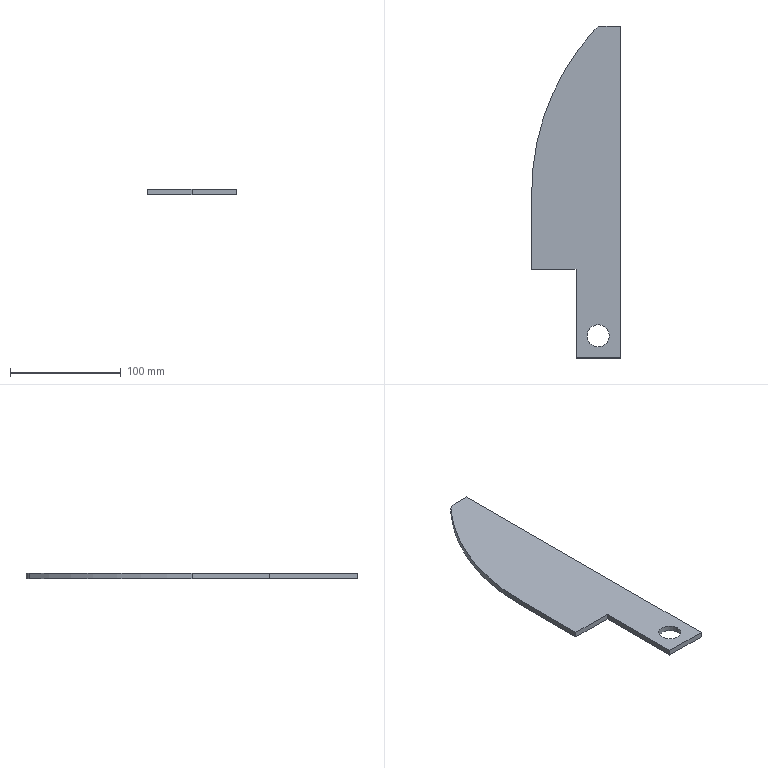Part | STEP file | qianjiaozheban | 1 solid | 11 faces | box 80 x 300 x 5 mm | volume 88356 mm3 | plane 8 | cylinder 3 | commonest cylinder face diameters 20 x2 435 x1
STEP:
#1=CARTESIAN_POINT('',(0.,0.,0.));
#2=DIRECTION('',(0.,0.,1.));
#3=DIRECTION('',(1.,0.,0.));
#4=AXIS2_PLACEMENT_3D('',#1,#2,#3);
#5=CARTESIAN_POINT('',(0.,80.,-2.5));
#6=VERTEX_POINT('',#5);
#7=CARTESIAN_POINT('',(0.,0.,-2.5));
#8=VERTEX_POINT('',#7);
#9=CARTESIAN_POINT('',(0.,0.,-2.5));
#10=DIRECTION('',(0.,-1.,0.));
#11=VECTOR('',#10,1.);
#12=LINE('',#9,#11);
#13=CARTESIAN_POINT('',(0.,0.,2.5));
#14=DIRECTION('',(1.,0.,0.));
#15=DIRECTION('',(0.,0.,-1.));
#16=AXIS2_PLACEMENT_3D('',#13,#14,#15);
#17=PLANE('',#16);
#18=CARTESIAN_POINT('',(5.,0.));
#19=DIRECTION('',(0.,-1.));
#20=VECTOR('',#19,1.);
#21=LINE('',#18,#20);
#22=(GEOMETRIC_REPRESENTATION_CONTEXT(2)PARAMETRIC_REPRESENTATION_CONTEXT()REPRESENTATION_CONTEXT('',''));
#23=DEFINITIONAL_REPRESENTATION('',(#21),#22);
#24=PCURVE('',#17,#23);
#25=CARTESIAN_POINT('',(177.5,150.,-2.5));
#26=DIRECTION('',(0.,0.,-1.));
#27=DIRECTION('',(-1.,0.,0.));
#28=AXIS2_PLACEMENT_3D('',#25,#26,#27);
#29=PLANE('',#28);
#30=CARTESIAN_POINT('',(177.5,-150.));
#31=DIRECTION('',(0.,-1.));
#32=VECTOR('',#31,1.);
#33=LINE('',#30,#32);
#34=(GEOMETRIC_REPRESENTATION_CONTEXT(2)PARAMETRIC_REPRESENTATION_CONTEXT()REPRESENTATION_CONTEXT('',''));
#35=DEFINITIONAL_REPRESENTATION('',(#33),#34);
#36=PCURVE('',#29,#35);
#37=SURFACE_CURVE('',#12,(#24,#36),.PCURVE_S1.);
#38=EDGE_CURVE('',#6,#8,#37,.T.);
#39=ORIENTED_EDGE('',*,*,#38,.T.);
#40=CARTESIAN_POINT('',(0.,0.,2.5));
#41=VERTEX_POINT('',#40);
#42=CARTESIAN_POINT('',(0.,0.,2.5));
#43=DIRECTION('',(0.,0.,-1.));
#44=VECTOR('',#43,1.);
#45=LINE('',#42,#44);
#46=CARTESIAN_POINT('',(0.,0.));
#47=DIRECTION('',(1.,0.));
#48=VECTOR('',#47,1.);
#49=LINE('',#46,#48);
#50=(GEOMETRIC_REPRESENTATION_CONTEXT(2)PARAMETRIC_REPRESENTATION_CONTEXT()REPRESENTATION_CONTEXT('',''));
#51=DEFINITIONAL_REPRESENTATION('',(#49),#50);
#52=PCURVE('',#17,#51);
#53=CARTESIAN_POINT('',(0.,0.,2.5));
#54=DIRECTION('',(0.,1.,0.));
#55=DIRECTION('',(0.,0.,1.));
#56=AXIS2_PLACEMENT_3D('',#53,#54,#55);
#57=PLANE('',#56);
#58=CARTESIAN_POINT('',(0.,0.));
#59=DIRECTION('',(-1.,0.));
#60=VECTOR('',#59,1.);
#61=LINE('',#58,#60);
#62=(GEOMETRIC_REPRESENTATION_CONTEXT(2)PARAMETRIC_REPRESENTATION_CONTEXT()REPRESENTATION_CONTEXT('',''));
#63=DEFINITIONAL_REPRESENTATION('',(#61),#62);
#64=PCURVE('',#57,#63);
#65=SURFACE_CURVE('',#45,(#52,#64),.PCURVE_S1.);
#66=EDGE_CURVE('',#41,#8,#65,.T.);
#67=ORIENTED_EDGE('',*,*,#66,.F.);
#68=CARTESIAN_POINT('',(0.,80.,2.5));
#69=VERTEX_POINT('',#68);
#70=CARTESIAN_POINT('',(0.,0.,2.5));
#71=DIRECTION('',(0.,-1.,0.));
#72=VECTOR('',#71,1.);
#73=LINE('',#70,#72);
#74=CARTESIAN_POINT('',(0.,0.));
#75=DIRECTION('',(0.,-1.));
#76=VECTOR('',#75,1.);
#77=LINE('',#74,#76);
#78=(GEOMETRIC_REPRESENTATION_CONTEXT(2)PARAMETRIC_REPRESENTATION_CONTEXT()REPRESENTATION_CONTEXT('',''));
#79=DEFINITIONAL_REPRESENTATION('',(#77),#78);
#80=PCURVE('',#17,#79);
#81=CARTESIAN_POINT('',(177.5,150.,2.5));
#82=DIRECTION('',(0.,0.,-1.));
#83=DIRECTION('',(-1.,0.,0.));
#84=AXIS2_PLACEMENT_3D('',#81,#82,#83);
#85=PLANE('',#84);
#86=CARTESIAN_POINT('',(177.5,-150.));
#87=DIRECTION('',(0.,-1.));
#88=VECTOR('',#87,1.);
#89=LINE('',#86,#88);
#90=(GEOMETRIC_REPRESENTATION_CONTEXT(2)PARAMETRIC_REPRESENTATION_CONTEXT()REPRESENTATION_CONTEXT('',''));
#91=DEFINITIONAL_REPRESENTATION('',(#89),#90);
#92=PCURVE('',#85,#91);
#93=SURFACE_CURVE('',#73,(#80,#92),.PCURVE_S1.);
#94=EDGE_CURVE('',#69,#41,#93,.T.);
#95=ORIENTED_EDGE('',*,*,#94,.F.);
#96=CARTESIAN_POINT('',(0.,80.,2.5));
#97=DIRECTION('',(0.,0.,-1.));
#98=VECTOR('',#97,1.);
#99=LINE('',#96,#98);
#100=CARTESIAN_POINT('',(0.,80.));
#101=DIRECTION('',(1.,0.));
#102=VECTOR('',#101,1.);
#103=LINE('',#100,#102);
#104=(GEOMETRIC_REPRESENTATION_CONTEXT(2)PARAMETRIC_REPRESENTATION_CONTEXT()REPRESENTATION_CONTEXT('',''));
#105=DEFINITIONAL_REPRESENTATION('',(#103),#104);
#106=PCURVE('',#17,#105);
#107=CARTESIAN_POINT('',(0.,80.,2.5));
#108=DIRECTION('',(0.,1.,0.));
#109=DIRECTION('',(0.,0.,1.));
#110=AXIS2_PLACEMENT_3D('',#107,#108,#109);
#111=PLANE('',#110);
#112=CARTESIAN_POINT('',(0.,0.));
#113=DIRECTION('',(-1.,0.));
#114=VECTOR('',#113,1.);
#115=LINE('',#112,#114);
#116=(GEOMETRIC_REPRESENTATION_CONTEXT(2)PARAMETRIC_REPRESENTATION_CONTEXT()REPRESENTATION_CONTEXT('',''));
#117=DEFINITIONAL_REPRESENTATION('',(#115),#116);
#118=PCURVE('',#111,#117);
#119=SURFACE_CURVE('',#99,(#106,#118),.PCURVE_S1.);
#120=EDGE_CURVE('',#69,#6,#119,.T.);
#121=ORIENTED_EDGE('',*,*,#120,.T.);
#122=EDGE_LOOP('',(#39,#67,#95,#121));
#123=FACE_BOUND('',#122,.T.);
#124=ADVANCED_FACE('',(#123),#17,.F.);
#125=CARTESIAN_POINT('',(40.,0.,-2.5));
#126=VERTEX_POINT('',#125);
#127=CARTESIAN_POINT('',(0.,0.,-2.5));
#128=DIRECTION('',(1.,0.,0.));
#129=VECTOR('',#128,1.);
#130=LINE('',#127,#129);
#131=CARTESIAN_POINT('',(-5.,0.));
#132=DIRECTION('',(0.,1.));
#133=VECTOR('',#132,1.);
#134=LINE('',#131,#133);
#135=(GEOMETRIC_REPRESENTATION_CONTEXT(2)PARAMETRIC_REPRESENTATION_CONTEXT()REPRESENTATION_CONTEXT('',''));
#136=DEFINITIONAL_REPRESENTATION('',(#134),#135);
#137=PCURVE('',#57,#136);
#138=CARTESIAN_POINT('',(177.5,-150.));
#139=DIRECTION('',(-1.,0.));
#140=VECTOR('',#139,1.);
#141=LINE('',#138,#140);
#142=(GEOMETRIC_REPRESENTATION_CONTEXT(2)PARAMETRIC_REPRESENTATION_CONTEXT()REPRESENTATION_CONTEXT('',''));
#143=DEFINITIONAL_REPRESENTATION('',(#141),#142);
#144=PCURVE('',#29,#143);
#145=SURFACE_CURVE('',#130,(#137,#144),.PCURVE_S1.);
#146=EDGE_CURVE('',#8,#126,#145,.T.);
#147=ORIENTED_EDGE('',*,*,#146,.T.);
#148=CARTESIAN_POINT('',(40.,0.,2.5));
#149=VERTEX_POINT('',#148);
#150=CARTESIAN_POINT('',(40.,0.,2.5));
#151=DIRECTION('',(0.,0.,-1.));
#152=VECTOR('',#151,1.);
#153=LINE('',#150,#152);
#154=CARTESIAN_POINT('',(0.,40.));
#155=DIRECTION('',(-1.,0.));
#156=VECTOR('',#155,1.);
#157=LINE('',#154,#156);
#158=(GEOMETRIC_REPRESENTATION_CONTEXT(2)PARAMETRIC_REPRESENTATION_CONTEXT()REPRESENTATION_CONTEXT('',''));
#159=DEFINITIONAL_REPRESENTATION('',(#157),#158);
#160=PCURVE('',#57,#159);
#161=CARTESIAN_POINT('',(40.,0.,2.5));
#162=DIRECTION('',(-1.,0.,0.));
#163=DIRECTION('',(0.,0.,1.));
#164=AXIS2_PLACEMENT_3D('',#161,#162,#163);
#165=PLANE('',#164);
#166=CARTESIAN_POINT('',(0.,0.));
#167=DIRECTION('',(-1.,0.));
#168=VECTOR('',#167,1.);
#169=LINE('',#166,#168);
#170=(GEOMETRIC_REPRESENTATION_CONTEXT(2)PARAMETRIC_REPRESENTATION_CONTEXT()REPRESENTATION_CONTEXT('',''));
#171=DEFINITIONAL_REPRESENTATION('',(#169),#170);
#172=PCURVE('',#165,#171);
#173=SURFACE_CURVE('',#153,(#160,#172),.PCURVE_S1.);
#174=EDGE_CURVE('',#149,#126,#173,.T.);
#175=ORIENTED_EDGE('',*,*,#174,.F.);
#176=CARTESIAN_POINT('',(0.,0.,2.5));
#177=DIRECTION('',(1.,0.,0.));
#178=VECTOR('',#177,1.);
#179=LINE('',#176,#178);
#180=CARTESIAN_POINT('',(0.,0.));
#181=DIRECTION('',(0.,1.));
#182=VECTOR('',#181,1.);
#183=LINE('',#180,#182);
#184=(GEOMETRIC_REPRESENTATION_CONTEXT(2)PARAMETRIC_REPRESENTATION_CONTEXT()REPRESENTATION_CONTEXT('',''));
#185=DEFINITIONAL_REPRESENTATION('',(#183),#184);
#186=PCURVE('',#57,#185);
#187=CARTESIAN_POINT('',(177.5,-150.));
#188=DIRECTION('',(-1.,0.));
#189=VECTOR('',#188,1.);
#190=LINE('',#187,#189);
#191=(GEOMETRIC_REPRESENTATION_CONTEXT(2)PARAMETRIC_REPRESENTATION_CONTEXT()REPRESENTATION_CONTEXT('',''));
#192=DEFINITIONAL_REPRESENTATION('',(#190),#191);
#193=PCURVE('',#85,#192);
#194=SURFACE_CURVE('',#179,(#186,#193),.PCURVE_S1.);
#195=EDGE_CURVE('',#41,#149,#194,.T.);
#196=ORIENTED_EDGE('',*,*,#195,.F.);
#197=ORIENTED_EDGE('',*,*,#66,.T.);
#198=EDGE_LOOP('',(#147,#175,#196,#197));
#199=FACE_BOUND('',#198,.T.);
#200=ADVANCED_FACE('',(#199),#57,.F.);
#201=CARTESIAN_POINT('',(40.,300.,-2.5));
#202=VERTEX_POINT('',#201);
#203=CARTESIAN_POINT('',(40.,0.,-2.5));
#204=DIRECTION('',(0.,1.,0.));
#205=VECTOR('',#204,1.);
#206=LINE('',#203,#205);
#207=CARTESIAN_POINT('',(-5.,0.));
#208=DIRECTION('',(0.,1.));
#209=VECTOR('',#208,1.);
#210=LINE('',#207,#209);
#211=(GEOMETRIC_REPRESENTATION_CONTEXT(2)PARAMETRIC_REPRESENTATION_CONTEXT()REPRESENTATION_CONTEXT('',''));
#212=DEFINITIONAL_REPRESENTATION('',(#210),#211);
#213=PCURVE('',#165,#212);
#214=CARTESIAN_POINT('',(137.5,-150.));
#215=DIRECTION('',(0.,1.));
#216=VECTOR('',#215,1.);
#217=LINE('',#214,#216);
#218=(GEOMETRIC_REPRESENTATION_CONTEXT(2)PARAMETRIC_REPRESENTATION_CONTEXT()REPRESENTATION_CONTEXT('',''));
#219=DEFINITIONAL_REPRESENTATION('',(#217),#218);
#220=PCURVE('',#29,#219);
#221=SURFACE_CURVE('',#206,(#213,#220),.PCURVE_S1.);
#222=EDGE_CURVE('',#126,#202,#221,.T.);
#223=ORIENTED_EDGE('',*,*,#222,.T.);
#224=CARTESIAN_POINT('',(40.,300.,2.5));
#225=VERTEX_POINT('',#224);
#226=CARTESIAN_POINT('',(40.,300.,2.5));
#227=DIRECTION('',(0.,0.,-1.));
#228=VECTOR('',#227,1.);
#229=LINE('',#226,#228);
#230=CARTESIAN_POINT('',(0.,300.));
#231=DIRECTION('',(-1.,0.));
#232=VECTOR('',#231,1.);
#233=LINE('',#230,#232);
#234=(GEOMETRIC_REPRESENTATION_CONTEXT(2)PARAMETRIC_REPRESENTATION_CONTEXT()REPRESENTATION_CONTEXT('',''));
#235=DEFINITIONAL_REPRESENTATION('',(#233),#234);
#236=PCURVE('',#165,#235);
#237=CARTESIAN_POINT('',(40.,300.,2.5));
#238=DIRECTION('',(0.,-1.,0.));
#239=DIRECTION('',(0.,0.,-1.));
#240=AXIS2_PLACEMENT_3D('',#237,#238,#239);
#241=PLANE('',#240);
#242=CARTESIAN_POINT('',(0.,0.));
#243=DIRECTION('',(1.,0.));
#244=VECTOR('',#243,1.);
#245=LINE('',#242,#244);
#246=(GEOMETRIC_REPRESENTATION_CONTEXT(2)PARAMETRIC_REPRESENTATION_CONTEXT()REPRESENTATION_CONTEXT('',''));
#247=DEFINITIONAL_REPRESENTATION('',(#245),#246);
#248=PCURVE('',#241,#247);
#249=SURFACE_CURVE('',#229,(#236,#248),.PCURVE_S1.);
#250=EDGE_CURVE('',#225,#202,#249,.T.);
#251=ORIENTED_EDGE('',*,*,#250,.F.);
#252=CARTESIAN_POINT('',(40.,0.,2.5));
#253=DIRECTION('',(0.,1.,0.));
#254=VECTOR('',#253,1.);
#255=LINE('',#252,#254);
#256=CARTESIAN_POINT('',(0.,0.));
#257=DIRECTION('',(0.,1.));
#258=VECTOR('',#257,1.);
#259=LINE('',#256,#258);
#260=(GEOMETRIC_REPRESENTATION_CONTEXT(2)PARAMETRIC_REPRESENTATION_CONTEXT()REPRESENTATION_CONTEXT('',''));
#261=DEFINITIONAL_REPRESENTATION('',(#259),#260);
#262=PCURVE('',#165,#261);
#263=CARTESIAN_POINT('',(137.5,-150.));
#264=DIRECTION('',(0.,1.));
#265=VECTOR('',#264,1.);
#266=LINE('',#263,#265);
#267=(GEOMETRIC_REPRESENTATION_CONTEXT(2)PARAMETRIC_REPRESENTATION_CONTEXT()REPRESENTATION_CONTEXT('',''));
#268=DEFINITIONAL_REPRESENTATION('',(#266),#267);
#269=PCURVE('',#85,#268);
#270=SURFACE_CURVE('',#255,(#262,#269),.PCURVE_S1.);
#271=EDGE_CURVE('',#149,#225,#270,.T.);
#272=ORIENTED_EDGE('',*,*,#271,.F.);
#273=ORIENTED_EDGE('',*,*,#174,.T.);
#274=EDGE_LOOP('',(#223,#251,#272,#273));
#275=FACE_BOUND('',#274,.T.);
#276=ADVANCED_FACE('',(#275),#165,.F.);
#277=CARTESIAN_POINT('',(24.346,300.,-2.5));
#278=VERTEX_POINT('',#277);
#279=CARTESIAN_POINT('',(40.,300.,-2.5));
#280=DIRECTION('',(-1.,0.,0.));
#281=VECTOR('',#280,1.);
#282=LINE('',#279,#281);
#283=CARTESIAN_POINT('',(5.,0.));
#284=DIRECTION('',(0.,-1.));
#285=VECTOR('',#284,1.);
#286=LINE('',#283,#285);
#287=(GEOMETRIC_REPRESENTATION_CONTEXT(2)PARAMETRIC_REPRESENTATION_CONTEXT()REPRESENTATION_CONTEXT('',''));
#288=DEFINITIONAL_REPRESENTATION('',(#286),#287);
#289=PCURVE('',#241,#288);
#290=CARTESIAN_POINT('',(137.5,150.));
#291=DIRECTION('',(1.,0.));
#292=VECTOR('',#291,1.);
#293=LINE('',#290,#292);
#294=(GEOMETRIC_REPRESENTATION_CONTEXT(2)PARAMETRIC_REPRESENTATION_CONTEXT()REPRESENTATION_CONTEXT('',''));
#295=DEFINITIONAL_REPRESENTATION('',(#293),#294);
#296=PCURVE('',#29,#295);
#297=SURFACE_CURVE('',#282,(#289,#296),.PCURVE_S1.);
#298=EDGE_CURVE('',#202,#278,#297,.T.);
#299=ORIENTED_EDGE('',*,*,#298,.T.);
#300=CARTESIAN_POINT('',(24.346,300.,2.5));
#301=VERTEX_POINT('',#300);
#302=CARTESIAN_POINT('',(24.346,300.,2.5));
#303=DIRECTION('',(0.,0.,-1.));
#304=VECTOR('',#303,1.);
#305=LINE('',#302,#304);
#306=CARTESIAN_POINT('',(0.,-15.654));
#307=DIRECTION('',(1.,0.));
#308=VECTOR('',#307,1.);
#309=LINE('',#306,#308);
#310=(GEOMETRIC_REPRESENTATION_CONTEXT(2)PARAMETRIC_REPRESENTATION_CONTEXT()REPRESENTATION_CONTEXT('',''));
#311=DEFINITIONAL_REPRESENTATION('',(#309),#310);
#312=PCURVE('',#241,#311);
#313=CARTESIAN_POINT('',(24.346,290.,2.5));
#314=DIRECTION('',(0.,0.,-1.));
#315=DIRECTION('',(-1.,0.,0.));
#316=AXIS2_PLACEMENT_3D('',#313,#314,#315);
#317=CYLINDRICAL_SURFACE('',#316,10.);
#318=CARTESIAN_POINT('',(1.571,0.));
#319=DIRECTION('',(0.,1.));
#320=VECTOR('',#319,1.);
#321=LINE('',#318,#320);
#322=(GEOMETRIC_REPRESENTATION_CONTEXT(2)PARAMETRIC_REPRESENTATION_CONTEXT()REPRESENTATION_CONTEXT('',''));
#323=DEFINITIONAL_REPRESENTATION('',(#321),#322);
#324=PCURVE('',#317,#323);
#325=SURFACE_CURVE('',#305,(#312,#324),.PCURVE_S1.);
#326=EDGE_CURVE('',#301,#278,#325,.T.);
#327=ORIENTED_EDGE('',*,*,#326,.F.);
#328=CARTESIAN_POINT('',(40.,300.,2.5));
#329=DIRECTION('',(-1.,0.,0.));
#330=VECTOR('',#329,1.);
#331=LINE('',#328,#330);
#332=CARTESIAN_POINT('',(0.,0.));
#333=DIRECTION('',(0.,-1.));
#334=VECTOR('',#333,1.);
#335=LINE('',#332,#334);
#336=(GEOMETRIC_REPRESENTATION_CONTEXT(2)PARAMETRIC_REPRESENTATION_CONTEXT()REPRESENTATION_CONTEXT('',''));
#337=DEFINITIONAL_REPRESENTATION('',(#335),#336);
#338=PCURVE('',#241,#337);
#339=CARTESIAN_POINT('',(137.5,150.));
#340=DIRECTION('',(1.,0.));
#341=VECTOR('',#340,1.);
#342=LINE('',#339,#341);
#343=(GEOMETRIC_REPRESENTATION_CONTEXT(2)PARAMETRIC_REPRESENTATION_CONTEXT()REPRESENTATION_CONTEXT('',''));
#344=DEFINITIONAL_REPRESENTATION('',(#342),#343);
#345=PCURVE('',#85,#344);
#346=SURFACE_CURVE('',#331,(#338,#345),.PCURVE_S1.);
#347=EDGE_CURVE('',#225,#301,#346,.T.);
#348=ORIENTED_EDGE('',*,*,#347,.F.);
#349=ORIENTED_EDGE('',*,*,#250,.T.);
#350=EDGE_LOOP('',(#299,#327,#348,#349));
#351=FACE_BOUND('',#350,.T.);
#352=ADVANCED_FACE('',(#351),#241,.F.);
#353=CARTESIAN_POINT('',(16.965,296.747,-2.5));
#354=VERTEX_POINT('',#353);
#355=CARTESIAN_POINT('',(24.346,290.,-2.5));
#356=DIRECTION('',(0.,0.,1.));
#357=DIRECTION('',(1.,0.,0.));
#358=AXIS2_PLACEMENT_3D('',#355,#356,#357);
#359=CIRCLE('',#358,10.);
#360=CARTESIAN_POINT('',(3.142,5.));
#361=DIRECTION('',(-1.,0.));
#362=VECTOR('',#361,1.);
#363=LINE('',#360,#362);
#364=(GEOMETRIC_REPRESENTATION_CONTEXT(2)PARAMETRIC_REPRESENTATION_CONTEXT()REPRESENTATION_CONTEXT('',''));
#365=DEFINITIONAL_REPRESENTATION('',(#363),#364);
#366=PCURVE('',#317,#365);
#367=CARTESIAN_POINT('',(143.154,140.));
#368=CARTESIAN_POINT('',(143.154,157.321));
#369=CARTESIAN_POINT('',(158.154,148.66));
#370=CARTESIAN_POINT('',(173.154,140.));
#371=CARTESIAN_POINT('',(158.154,131.34));
#372=CARTESIAN_POINT('',(143.154,122.679));
#373=CARTESIAN_POINT('',(143.154,140.));
#374=(BOUNDED_CURVE()B_SPLINE_CURVE(2,(#367,#368,#369,#370,#371,#372,#373),.UNSPECIFIED.,.T.,.F.)B_SPLINE_CURVE_WITH_KNOTS((1,2,2,2,2,1),(-2.094,0.,2.094,4.189,6.283,8.378),.UNSPECIFIED.)CURVE()GEOMETRIC_REPRESENTATION_ITEM()RATIONAL_B_SPLINE_CURVE((1.,0.5,1.,0.5,1.,0.5,1.))REPRESENTATION_ITEM(''));
#375=(GEOMETRIC_REPRESENTATION_CONTEXT(2)PARAMETRIC_REPRESENTATION_CONTEXT()REPRESENTATION_CONTEXT('',''));
#376=DEFINITIONAL_REPRESENTATION('',(#374),#375);
#377=PCURVE('',#29,#376);
#378=SURFACE_CURVE('',#359,(#366,#377),.PCURVE_S1.);
#379=EDGE_CURVE('',#278,#354,#378,.T.);
#380=ORIENTED_EDGE('',*,*,#379,.T.);
#381=CARTESIAN_POINT('',(16.965,296.747,2.5));
#382=VERTEX_POINT('',#381);
#383=CARTESIAN_POINT('',(16.965,296.747,2.5));
#384=DIRECTION('',(0.,0.,-1.));
#385=VECTOR('',#384,1.);
#386=LINE('',#383,#385);
#387=CARTESIAN_POINT('',(0.7406,0.));
#388=DIRECTION('',(0.,1.));
#389=VECTOR('',#388,1.);
#390=LINE('',#387,#389);
#391=(GEOMETRIC_REPRESENTATION_CONTEXT(2)PARAMETRIC_REPRESENTATION_CONTEXT()REPRESENTATION_CONTEXT('',''));
#392=DEFINITIONAL_REPRESENTATION('',(#390),#391);
#393=PCURVE('',#317,#392);
#394=CARTESIAN_POINT('',(177.5,150.,2.5));
#395=DIRECTION('',(0.,0.,-1.));
#396=DIRECTION('',(-1.,0.,0.));
#397=AXIS2_PLACEMENT_3D('',#394,#395,#396);
#398=CYLINDRICAL_SURFACE('',#397,217.5);
#399=CARTESIAN_POINT('',(0.7406,0.));
#400=DIRECTION('',(0.,1.));
#401=VECTOR('',#400,1.);
#402=LINE('',#399,#401);
#403=(GEOMETRIC_REPRESENTATION_CONTEXT(2)PARAMETRIC_REPRESENTATION_CONTEXT()REPRESENTATION_CONTEXT('',''));
#404=DEFINITIONAL_REPRESENTATION('',(#402),#403);
#405=PCURVE('',#398,#404);
#406=SURFACE_CURVE('',#386,(#393,#405),.PCURVE_S1.);
#407=EDGE_CURVE('',#382,#354,#406,.T.);
#408=ORIENTED_EDGE('',*,*,#407,.F.);
#409=CARTESIAN_POINT('',(24.346,290.,2.5));
#410=DIRECTION('',(0.,0.,1.));
#411=DIRECTION('',(1.,0.,0.));
#412=AXIS2_PLACEMENT_3D('',#409,#410,#411);
#413=CIRCLE('',#412,10.);
#414=CARTESIAN_POINT('',(3.142,0.));
#415=DIRECTION('',(-1.,0.));
#416=VECTOR('',#415,1.);
#417=LINE('',#414,#416);
#418=(GEOMETRIC_REPRESENTATION_CONTEXT(2)PARAMETRIC_REPRESENTATION_CONTEXT()REPRESENTATION_CONTEXT('',''));
#419=DEFINITIONAL_REPRESENTATION('',(#417),#418);
#420=PCURVE('',#317,#419);
#421=CARTESIAN_POINT('',(143.154,140.));
#422=CARTESIAN_POINT('',(143.154,157.321));
#423=CARTESIAN_POINT('',(158.154,148.66));
#424=CARTESIAN_POINT('',(173.154,140.));
#425=CARTESIAN_POINT('',(158.154,131.34));
#426=CARTESIAN_POINT('',(143.154,122.679));
#427=CARTESIAN_POINT('',(143.154,140.));
#428=(BOUNDED_CURVE()B_SPLINE_CURVE(2,(#421,#422,#423,#424,#425,#426,#427),.UNSPECIFIED.,.T.,.F.)B_SPLINE_CURVE_WITH_KNOTS((1,2,2,2,2,1),(-2.094,0.,2.094,4.189,6.283,8.378),.UNSPECIFIED.)CURVE()GEOMETRIC_REPRESENTATION_ITEM()RATIONAL_B_SPLINE_CURVE((1.,0.5,1.,0.5,1.,0.5,1.))REPRESENTATION_ITEM(''));
#429=(GEOMETRIC_REPRESENTATION_CONTEXT(2)PARAMETRIC_REPRESENTATION_CONTEXT()REPRESENTATION_CONTEXT('',''));
#430=DEFINITIONAL_REPRESENTATION('',(#428),#429);
#431=PCURVE('',#85,#430);
#432=SURFACE_CURVE('',#413,(#420,#431),.PCURVE_S1.);
#433=EDGE_CURVE('',#301,#382,#432,.T.);
#434=ORIENTED_EDGE('',*,*,#433,.F.);
#435=ORIENTED_EDGE('',*,*,#326,.T.);
#436=EDGE_LOOP('',(#380,#408,#434,#435));
#437=FACE_BOUND('',#436,.T.);
#438=ADVANCED_FACE('',(#437),#317,.T.);
#439=CARTESIAN_POINT('',(-40.,150.,-2.5));
#440=VERTEX_POINT('',#439);
#441=CARTESIAN_POINT('',(177.5,150.,-2.5));
#442=DIRECTION('',(0.,0.,1.));
#443=DIRECTION('',(-1.,0.,0.));
#444=AXIS2_PLACEMENT_3D('',#441,#442,#443);
#445=CIRCLE('',#444,217.5);
#446=CARTESIAN_POINT('',(6.283,5.));
#447=DIRECTION('',(-1.,0.));
#448=VECTOR('',#447,1.);
#449=LINE('',#446,#448);
#450=(GEOMETRIC_REPRESENTATION_CONTEXT(2)PARAMETRIC_REPRESENTATION_CONTEXT()REPRESENTATION_CONTEXT('',''));
#451=DEFINITIONAL_REPRESENTATION('',(#449),#450);
#452=PCURVE('',#398,#451);
#453=CARTESIAN_POINT('',(217.5,0.));
#454=CARTESIAN_POINT('',(217.5,-376.721));
#455=CARTESIAN_POINT('',(-108.75,-188.361));
#456=CARTESIAN_POINT('',(-435.,0.));
#457=CARTESIAN_POINT('',(-108.75,188.361));
#458=CARTESIAN_POINT('',(217.5,376.721));
#459=CARTESIAN_POINT('',(217.5,0.));
#460=(BOUNDED_CURVE()B_SPLINE_CURVE(2,(#453,#454,#455,#456,#457,#458,#459),.UNSPECIFIED.,.T.,.F.)B_SPLINE_CURVE_WITH_KNOTS((1,2,2,2,2,1),(-2.094,0.,2.094,4.189,6.283,8.378),.UNSPECIFIED.)CURVE()GEOMETRIC_REPRESENTATION_ITEM()RATIONAL_B_SPLINE_CURVE((1.,0.5,1.,0.5,1.,0.5,1.))REPRESENTATION_ITEM(''));
#461=(GEOMETRIC_REPRESENTATION_CONTEXT(2)PARAMETRIC_REPRESENTATION_CONTEXT()REPRESENTATION_CONTEXT('',''));
#462=DEFINITIONAL_REPRESENTATION('',(#460),#461);
#463=PCURVE('',#29,#462);
#464=SURFACE_CURVE('',#445,(#452,#463),.PCURVE_S1.);
#465=EDGE_CURVE('',#354,#440,#464,.T.);
#466=ORIENTED_EDGE('',*,*,#465,.T.);
#467=CARTESIAN_POINT('',(-40.,150.,2.5));
#468=VERTEX_POINT('',#467);
#469=CARTESIAN_POINT('',(-40.,150.,2.5));
#470=DIRECTION('',(0.,0.,-1.));
#471=VECTOR('',#470,1.);
#472=LINE('',#469,#471);
#473=CARTESIAN_POINT('',(0.,0.));
#474=DIRECTION('',(0.,1.));
#475=VECTOR('',#474,1.);
#476=LINE('',#473,#475);
#477=(GEOMETRIC_REPRESENTATION_CONTEXT(2)PARAMETRIC_REPRESENTATION_CONTEXT()REPRESENTATION_CONTEXT('',''));
#478=DEFINITIONAL_REPRESENTATION('',(#476),#477);
#479=PCURVE('',#398,#478);
#480=CARTESIAN_POINT('',(-40.,80.,2.5));
#481=DIRECTION('',(1.,0.,0.));
#482=DIRECTION('',(0.,0.,-1.));
#483=AXIS2_PLACEMENT_3D('',#480,#481,#482);
#484=PLANE('',#483);
#485=CARTESIAN_POINT('',(0.,70.));
#486=DIRECTION('',(1.,0.));
#487=VECTOR('',#486,1.);
#488=LINE('',#485,#487);
#489=(GEOMETRIC_REPRESENTATION_CONTEXT(2)PARAMETRIC_REPRESENTATION_CONTEXT()REPRESENTATION_CONTEXT('',''));
#490=DEFINITIONAL_REPRESENTATION('',(#488),#489);
#491=PCURVE('',#484,#490);
#492=SURFACE_CURVE('',#472,(#479,#491),.PCURVE_S1.);
#493=EDGE_CURVE('',#468,#440,#492,.T.);
#494=ORIENTED_EDGE('',*,*,#493,.F.);
#495=CARTESIAN_POINT('',(177.5,150.,2.5));
#496=DIRECTION('',(0.,0.,1.));
#497=DIRECTION('',(-1.,0.,0.));
#498=AXIS2_PLACEMENT_3D('',#495,#496,#497);
#499=CIRCLE('',#498,217.5);
#500=CARTESIAN_POINT('',(6.283,0.));
#501=DIRECTION('',(-1.,0.));
#502=VECTOR('',#501,1.);
#503=LINE('',#500,#502);
#504=(GEOMETRIC_REPRESENTATION_CONTEXT(2)PARAMETRIC_REPRESENTATION_CONTEXT()REPRESENTATION_CONTEXT('',''));
#505=DEFINITIONAL_REPRESENTATION('',(#503),#504);
#506=PCURVE('',#398,#505);
#507=CARTESIAN_POINT('',(217.5,0.));
#508=CARTESIAN_POINT('',(217.5,-376.721));
#509=CARTESIAN_POINT('',(-108.75,-188.361));
#510=CARTESIAN_POINT('',(-435.,0.));
#511=CARTESIAN_POINT('',(-108.75,188.361));
#512=CARTESIAN_POINT('',(217.5,376.721));
#513=CARTESIAN_POINT('',(217.5,0.));
#514=(BOUNDED_CURVE()B_SPLINE_CURVE(2,(#507,#508,#509,#510,#511,#512,#513),.UNSPECIFIED.,.T.,.F.)B_SPLINE_CURVE_WITH_KNOTS((1,2,2,2,2,1),(-2.094,0.,2.094,4.189,6.283,8.378),.UNSPECIFIED.)CURVE()GEOMETRIC_REPRESENTATION_ITEM()RATIONAL_B_SPLINE_CURVE((1.,0.5,1.,0.5,1.,0.5,1.))REPRESENTATION_ITEM(''));
#515=(GEOMETRIC_REPRESENTATION_CONTEXT(2)PARAMETRIC_REPRESENTATION_CONTEXT()REPRESENTATION_CONTEXT('',''));
#516=DEFINITIONAL_REPRESENTATION('',(#514),#515);
#517=PCURVE('',#85,#516);
#518=SURFACE_CURVE('',#499,(#506,#517),.PCURVE_S1.);
#519=EDGE_CURVE('',#382,#468,#518,.T.);
#520=ORIENTED_EDGE('',*,*,#519,.F.);
#521=ORIENTED_EDGE('',*,*,#407,.T.);
#522=EDGE_LOOP('',(#466,#494,#520,#521));
#523=FACE_BOUND('',#522,.T.);
#524=ADVANCED_FACE('',(#523),#398,.T.);
#525=CARTESIAN_POINT('',(-40.,80.,-2.5));
#526=VERTEX_POINT('',#525);
#527=CARTESIAN_POINT('',(-40.,80.,-2.5));
#528=DIRECTION('',(0.,-1.,0.));
#529=VECTOR('',#528,1.);
#530=LINE('',#527,#529);
#531=CARTESIAN_POINT('',(5.,0.));
#532=DIRECTION('',(0.,-1.));
#533=VECTOR('',#532,1.);
#534=LINE('',#531,#533);
#535=(GEOMETRIC_REPRESENTATION_CONTEXT(2)PARAMETRIC_REPRESENTATION_CONTEXT()REPRESENTATION_CONTEXT('',''));
#536=DEFINITIONAL_REPRESENTATION('',(#534),#535);
#537=PCURVE('',#484,#536);
#538=CARTESIAN_POINT('',(217.5,-70.));
#539=DIRECTION('',(0.,-1.));
#540=VECTOR('',#539,1.);
#541=LINE('',#538,#540);
#542=(GEOMETRIC_REPRESENTATION_CONTEXT(2)PARAMETRIC_REPRESENTATION_CONTEXT()REPRESENTATION_CONTEXT('',''));
#543=DEFINITIONAL_REPRESENTATION('',(#541),#542);
#544=PCURVE('',#29,#543);
#545=SURFACE_CURVE('',#530,(#537,#544),.PCURVE_S1.);
#546=EDGE_CURVE('',#440,#526,#545,.T.);
#547=ORIENTED_EDGE('',*,*,#546,.T.);
#548=CARTESIAN_POINT('',(-40.,80.,2.5));
#549=VERTEX_POINT('',#548);
#550=CARTESIAN_POINT('',(-40.,80.,2.5));
#551=DIRECTION('',(0.,0.,-1.));
#552=VECTOR('',#551,1.);
#553=LINE('',#550,#552);
#554=CARTESIAN_POINT('',(0.,0.));
#555=DIRECTION('',(1.,0.));
#556=VECTOR('',#555,1.);
#557=LINE('',#554,#556);
#558=(GEOMETRIC_REPRESENTATION_CONTEXT(2)PARAMETRIC_REPRESENTATION_CONTEXT()REPRESENTATION_CONTEXT('',''));
#559=DEFINITIONAL_REPRESENTATION('',(#557),#558);
#560=PCURVE('',#484,#559);
#561=CARTESIAN_POINT('',(0.,-40.));
#562=DIRECTION('',(-1.,0.));
#563=VECTOR('',#562,1.);
#564=LINE('',#561,#563);
#565=(GEOMETRIC_REPRESENTATION_CONTEXT(2)PARAMETRIC_REPRESENTATION_CONTEXT()REPRESENTATION_CONTEXT('',''));
#566=DEFINITIONAL_REPRESENTATION('',(#564),#565);
#567=PCURVE('',#111,#566);
#568=SURFACE_CURVE('',#553,(#560,#567),.PCURVE_S1.);
#569=EDGE_CURVE('',#549,#526,#568,.T.);
#570=ORIENTED_EDGE('',*,*,#569,.F.);
#571=CARTESIAN_POINT('',(-40.,80.,2.5));
#572=DIRECTION('',(0.,-1.,0.));
#573=VECTOR('',#572,1.);
#574=LINE('',#571,#573);
#575=CARTESIAN_POINT('',(0.,0.));
#576=DIRECTION('',(0.,-1.));
#577=VECTOR('',#576,1.);
#578=LINE('',#575,#577);
#579=(GEOMETRIC_REPRESENTATION_CONTEXT(2)PARAMETRIC_REPRESENTATION_CONTEXT()REPRESENTATION_CONTEXT('',''));
#580=DEFINITIONAL_REPRESENTATION('',(#578),#579);
#581=PCURVE('',#484,#580);
#582=CARTESIAN_POINT('',(217.5,-70.));
#583=DIRECTION('',(0.,-1.));
#584=VECTOR('',#583,1.);
#585=LINE('',#582,#584);
#586=(GEOMETRIC_REPRESENTATION_CONTEXT(2)PARAMETRIC_REPRESENTATION_CONTEXT()REPRESENTATION_CONTEXT('',''));
#587=DEFINITIONAL_REPRESENTATION('',(#585),#586);
#588=PCURVE('',#85,#587);
#589=SURFACE_CURVE('',#574,(#581,#588),.PCURVE_S1.);
#590=EDGE_CURVE('',#468,#549,#589,.T.);
#591=ORIENTED_EDGE('',*,*,#590,.F.);
#592=ORIENTED_EDGE('',*,*,#493,.T.);
#593=EDGE_LOOP('',(#547,#570,#591,#592));
#594=FACE_BOUND('',#593,.T.);
#595=ADVANCED_FACE('',(#594),#484,.F.);
#596=CARTESIAN_POINT('',(0.,80.,-2.5));
#597=DIRECTION('',(1.,0.,0.));
#598=VECTOR('',#597,1.);
#599=LINE('',#596,#598);
#600=CARTESIAN_POINT('',(-5.,0.));
#601=DIRECTION('',(0.,1.));
#602=VECTOR('',#601,1.);
#603=LINE('',#600,#602);
#604=(GEOMETRIC_REPRESENTATION_CONTEXT(2)PARAMETRIC_REPRESENTATION_CONTEXT()REPRESENTATION_CONTEXT('',''));
#605=DEFINITIONAL_REPRESENTATION('',(#603),#604);
#606=PCURVE('',#111,#605);
#607=CARTESIAN_POINT('',(177.5,-70.));
#608=DIRECTION('',(-1.,0.));
#609=VECTOR('',#608,1.);
#610=LINE('',#607,#609);
#611=(GEOMETRIC_REPRESENTATION_CONTEXT(2)PARAMETRIC_REPRESENTATION_CONTEXT()REPRESENTATION_CONTEXT('',''));
#612=DEFINITIONAL_REPRESENTATION('',(#610),#611);
#613=PCURVE('',#29,#612);
#614=SURFACE_CURVE('',#599,(#606,#613),.PCURVE_S1.);
#615=EDGE_CURVE('',#526,#6,#614,.T.);
#616=ORIENTED_EDGE('',*,*,#615,.T.);
#617=ORIENTED_EDGE('',*,*,#120,.F.);
#618=CARTESIAN_POINT('',(0.,80.,2.5));
#619=DIRECTION('',(1.,0.,0.));
#620=VECTOR('',#619,1.);
#621=LINE('',#618,#620);
#622=CARTESIAN_POINT('',(0.,0.));
#623=DIRECTION('',(0.,1.));
#624=VECTOR('',#623,1.);
#625=LINE('',#622,#624);
#626=(GEOMETRIC_REPRESENTATION_CONTEXT(2)PARAMETRIC_REPRESENTATION_CONTEXT()REPRESENTATION_CONTEXT('',''));
#627=DEFINITIONAL_REPRESENTATION('',(#625),#626);
#628=PCURVE('',#111,#627);
#629=CARTESIAN_POINT('',(177.5,-70.));
#630=DIRECTION('',(-1.,0.));
#631=VECTOR('',#630,1.);
#632=LINE('',#629,#631);
#633=(GEOMETRIC_REPRESENTATION_CONTEXT(2)PARAMETRIC_REPRESENTATION_CONTEXT()REPRESENTATION_CONTEXT('',''));
#634=DEFINITIONAL_REPRESENTATION('',(#632),#633);
#635=PCURVE('',#85,#634);
#636=SURFACE_CURVE('',#621,(#628,#635),.PCURVE_S1.);
#637=EDGE_CURVE('',#549,#69,#636,.T.);
#638=ORIENTED_EDGE('',*,*,#637,.F.);
#639=ORIENTED_EDGE('',*,*,#569,.T.);
#640=EDGE_LOOP('',(#616,#617,#638,#639));
#641=FACE_BOUND('',#640,.T.);
#642=ADVANCED_FACE('',(#641),#111,.F.);
#643=CARTESIAN_POINT('',(30.,20.,2.5));
#644=VERTEX_POINT('',#643);
#645=CARTESIAN_POINT('',(20.,20.,2.5));
#646=DIRECTION('',(0.,0.,1.));
#647=DIRECTION('',(1.,0.,0.));
#648=AXIS2_PLACEMENT_3D('',#645,#646,#647);
#649=CIRCLE('',#648,10.);
#650=CARTESIAN_POINT('',(147.5,-130.));
#651=CARTESIAN_POINT('',(147.5,-112.679));
#652=CARTESIAN_POINT('',(162.5,-121.34));
#653=CARTESIAN_POINT('',(177.5,-130.));
#654=CARTESIAN_POINT('',(162.5,-138.66));
#655=CARTESIAN_POINT('',(147.5,-147.321));
#656=CARTESIAN_POINT('',(147.5,-130.));
#657=(BOUNDED_CURVE()B_SPLINE_CURVE(2,(#650,#651,#652,#653,#654,#655,#656),.UNSPECIFIED.,.T.,.F.)B_SPLINE_CURVE_WITH_KNOTS((1,2,2,2,2,1),(-2.094,0.,2.094,4.189,6.283,8.378),.UNSPECIFIED.)CURVE()GEOMETRIC_REPRESENTATION_ITEM()RATIONAL_B_SPLINE_CURVE((1.,0.5,1.,0.5,1.,0.5,1.))REPRESENTATION_ITEM(''));
#658=(GEOMETRIC_REPRESENTATION_CONTEXT(2)PARAMETRIC_REPRESENTATION_CONTEXT()REPRESENTATION_CONTEXT('',''));
#659=DEFINITIONAL_REPRESENTATION('',(#657),#658);
#660=PCURVE('',#85,#659);
#661=CARTESIAN_POINT('',(20.,20.,-2.5));
#662=DIRECTION('',(0.,0.,1.));
#663=DIRECTION('',(1.,0.,0.));
#664=AXIS2_PLACEMENT_3D('',#661,#662,#663);
#665=CYLINDRICAL_SURFACE('',#664,10.);
#666=CARTESIAN_POINT('',(0.,5.));
#667=DIRECTION('',(1.,0.));
#668=VECTOR('',#667,1.);
#669=LINE('',#666,#668);
#670=(GEOMETRIC_REPRESENTATION_CONTEXT(2)PARAMETRIC_REPRESENTATION_CONTEXT()REPRESENTATION_CONTEXT('',''));
#671=DEFINITIONAL_REPRESENTATION('',(#669),#670);
#672=PCURVE('',#665,#671);
#673=SURFACE_CURVE('',#649,(#660,#672),.PCURVE_S1.);
#674=EDGE_CURVE('',#644,#644,#673,.T.);
#675=ORIENTED_EDGE('',*,*,#674,.F.);
#676=EDGE_LOOP('',(#675));
#677=FACE_BOUND('',#676,.T.);
#678=ORIENTED_EDGE('',*,*,#94,.T.);
#679=ORIENTED_EDGE('',*,*,#195,.T.);
#680=ORIENTED_EDGE('',*,*,#271,.T.);
#681=ORIENTED_EDGE('',*,*,#347,.T.);
#682=ORIENTED_EDGE('',*,*,#433,.T.);
#683=ORIENTED_EDGE('',*,*,#519,.T.);
#684=ORIENTED_EDGE('',*,*,#590,.T.);
#685=ORIENTED_EDGE('',*,*,#637,.T.);
#686=EDGE_LOOP('',(#678,#679,#680,#681,#682,#683,#684,#685));
#687=FACE_BOUND('',#686,.T.);
#688=ADVANCED_FACE('',(#677,#687),#85,.F.);
#689=CARTESIAN_POINT('',(30.,20.,-2.5));
#690=VERTEX_POINT('',#689);
#691=CARTESIAN_POINT('',(20.,20.,-2.5));
#692=DIRECTION('',(0.,0.,1.));
#693=DIRECTION('',(1.,0.,0.));
#694=AXIS2_PLACEMENT_3D('',#691,#692,#693);
#695=CIRCLE('',#694,10.);
#696=CARTESIAN_POINT('',(147.5,-130.));
#697=CARTESIAN_POINT('',(147.5,-112.679));
#698=CARTESIAN_POINT('',(162.5,-121.34));
#699=CARTESIAN_POINT('',(177.5,-130.));
#700=CARTESIAN_POINT('',(162.5,-138.66));
#701=CARTESIAN_POINT('',(147.5,-147.321));
#702=CARTESIAN_POINT('',(147.5,-130.));
#703=(BOUNDED_CURVE()B_SPLINE_CURVE(2,(#696,#697,#698,#699,#700,#701,#702),.UNSPECIFIED.,.T.,.F.)B_SPLINE_CURVE_WITH_KNOTS((1,2,2,2,2,1),(-2.094,0.,2.094,4.189,6.283,8.378),.UNSPECIFIED.)CURVE()GEOMETRIC_REPRESENTATION_ITEM()RATIONAL_B_SPLINE_CURVE((1.,0.5,1.,0.5,1.,0.5,1.))REPRESENTATION_ITEM(''));
#704=(GEOMETRIC_REPRESENTATION_CONTEXT(2)PARAMETRIC_REPRESENTATION_CONTEXT()REPRESENTATION_CONTEXT('',''));
#705=DEFINITIONAL_REPRESENTATION('',(#703),#704);
#706=PCURVE('',#29,#705);
#707=CARTESIAN_POINT('',(0.,0.));
#708=DIRECTION('',(1.,0.));
#709=VECTOR('',#708,1.);
#710=LINE('',#707,#709);
#711=(GEOMETRIC_REPRESENTATION_CONTEXT(2)PARAMETRIC_REPRESENTATION_CONTEXT()REPRESENTATION_CONTEXT('',''));
#712=DEFINITIONAL_REPRESENTATION('',(#710),#711);
#713=PCURVE('',#665,#712);
#714=SURFACE_CURVE('',#695,(#706,#713),.PCURVE_S1.);
#715=EDGE_CURVE('',#690,#690,#714,.T.);
#716=ORIENTED_EDGE('',*,*,#715,.T.);
#717=EDGE_LOOP('',(#716));
#718=FACE_BOUND('',#717,.T.);
#719=ORIENTED_EDGE('',*,*,#38,.F.);
#720=ORIENTED_EDGE('',*,*,#615,.F.);
#721=ORIENTED_EDGE('',*,*,#546,.F.);
#722=ORIENTED_EDGE('',*,*,#465,.F.);
#723=ORIENTED_EDGE('',*,*,#379,.F.);
#724=ORIENTED_EDGE('',*,*,#298,.F.);
#725=ORIENTED_EDGE('',*,*,#222,.F.);
#726=ORIENTED_EDGE('',*,*,#146,.F.);
#727=EDGE_LOOP('',(#719,#720,#721,#722,#723,#724,#725,#726));
#728=FACE_BOUND('',#727,.T.);
#729=ADVANCED_FACE('',(#718,#728),#29,.T.);
#730=ORIENTED_EDGE('',*,*,#715,.T.);
#731=CARTESIAN_POINT('',(30.,20.,-2.5));
#732=CARTESIAN_POINT('',(30.,20.,2.5));
#733=B_SPLINE_CURVE_WITH_KNOTS('',1,(#731,#732),.UNSPECIFIED.,.F.,.F.,(2,2),(0.,5.),.PIECEWISE_BEZIER_KNOTS.);
#734=CARTESIAN_POINT('',(6.283,0.));
#735=DIRECTION('',(0.,1.));
#736=VECTOR('',#735,1.);
#737=LINE('',#734,#736);
#738=(GEOMETRIC_REPRESENTATION_CONTEXT(2)PARAMETRIC_REPRESENTATION_CONTEXT()REPRESENTATION_CONTEXT('',''));
#739=DEFINITIONAL_REPRESENTATION('',(#737),#738);
#740=PCURVE('',#665,#739);
#741=CARTESIAN_POINT('',(0.,0.));
#742=DIRECTION('',(0.,1.));
#743=VECTOR('',#742,1.);
#744=LINE('',#741,#743);
#745=(GEOMETRIC_REPRESENTATION_CONTEXT(2)PARAMETRIC_REPRESENTATION_CONTEXT()REPRESENTATION_CONTEXT('',''));
#746=DEFINITIONAL_REPRESENTATION('',(#744),#745);
#747=PCURVE('',#665,#746);
#748=SEAM_CURVE('',#733,(#740,#747),.PCURVE_S1.);
#749=EDGE_CURVE('',#690,#644,#748,.T.);
#750=ORIENTED_EDGE('',*,*,#749,.T.);
#751=ORIENTED_EDGE('',*,*,#674,.F.);
#752=ORIENTED_EDGE('',*,*,#749,.F.);
#753=EDGE_LOOP('',(#730,#750,#751,#752));
#754=FACE_BOUND('',#753,.F.);
#755=ADVANCED_FACE('',(#754),#665,.F.);
#756=CLOSED_SHELL('',(#124,#200,#276,#352,#438,#524,#595,#642,#688,#729,#755));
#757=MANIFOLD_SOLID_BREP('',#756);
#758=(LENGTH_UNIT()NAMED_UNIT(*)SI_UNIT(.MILLI.,.METRE.));
#759=UNCERTAINTY_MEASURE_WITH_UNIT(LENGTH_MEASURE(0.000001),#758,'','');
#760=(NAMED_UNIT(*)PLANE_ANGLE_UNIT()SI_UNIT($,.RADIAN.));
#761=(NAMED_UNIT(*)SI_UNIT($,.STERADIAN.)SOLID_ANGLE_UNIT());
#762=(GEOMETRIC_REPRESENTATION_CONTEXT(3)GLOBAL_UNCERTAINTY_ASSIGNED_CONTEXT((#759))GLOBAL_UNIT_ASSIGNED_CONTEXT((#758,#760,#761))REPRESENTATION_CONTEXT('',''));
#763=ADVANCED_BREP_SHAPE_REPRESENTATION('',(#4,#757),#762);